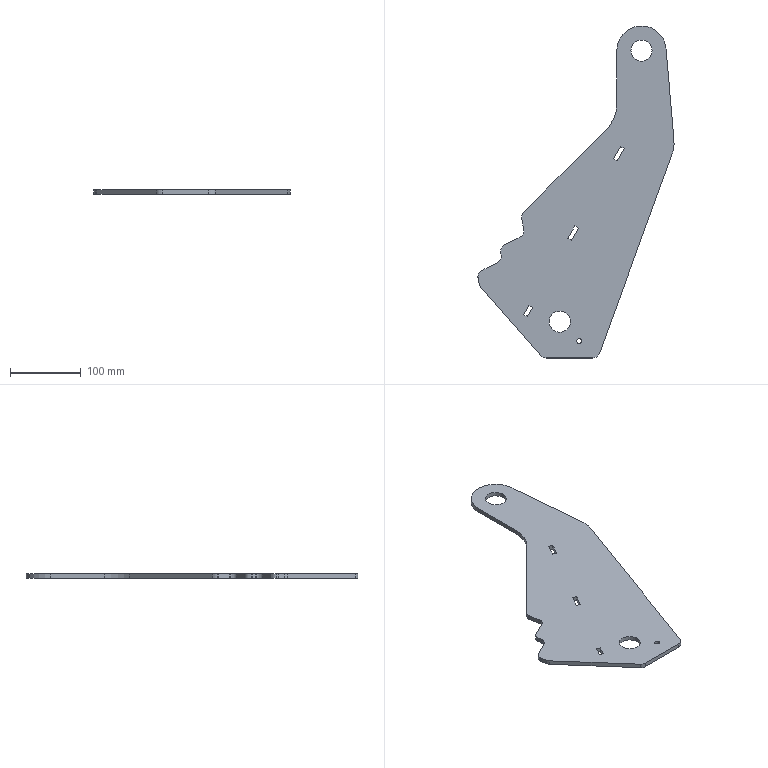Part | SolidWorks | features Fillet 2, FlatPattern 1, HoleWzd 1, SMBaseFlange 1, SheetMetal 1 | 1 solid | 48 faces | box 278.099 x 471.04 x 6 mm | volume 357826 mm3 | plane 25 | cylinder 23 | commonest cylinder face diameters 20 x14 30 x4 6.8 x2 100 x2 70 x1